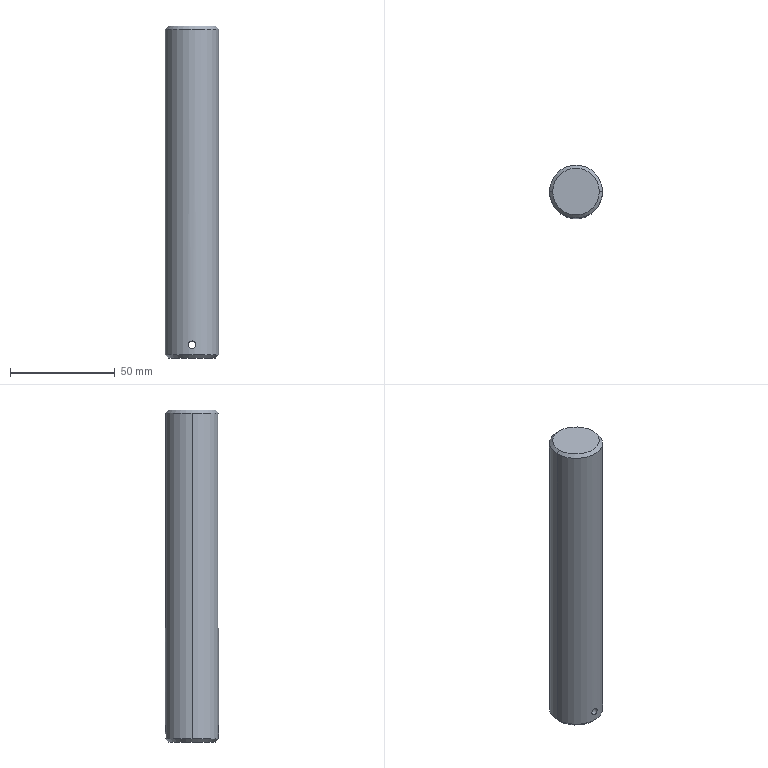Part | SolidWorks | features Chamfer 1, Extrusion 1, ICE 1 | 1 solid | 10 faces | box 25.4 x 25.4 x 158.75 mm | volume 80008 mm3 | cylinder 4 | cone 4 | plane 2 | commonest cylinder face diameters 3.57 x2 25.4 x2
STEP:
#1=CARTESIAN_POINT('',(0.,-12.7,4.565));
#2=VERTEX_POINT('',#1);
#3=CARTESIAN_POINT('',(0.,-12.7,8.135));
#4=VERTEX_POINT('',#3);
#5=CARTESIAN_POINT('',(0.,-12.7,4.565));
#6=CARTESIAN_POINT('',(-0.2331,-12.7,4.565));
#7=CARTESIAN_POINT('',(-0.4682,-12.693,4.612));
#8=CARTESIAN_POINT('',(-0.8979,-12.67,4.79));
#9=CARTESIAN_POINT('',(-1.097,-12.654,4.923));
#10=CARTESIAN_POINT('',(-1.344,-12.629,5.169));
#11=CARTESIAN_POINT('',(-1.419,-12.621,5.261));
#12=CARTESIAN_POINT('',(-1.549,-12.605,5.455));
#13=CARTESIAN_POINT('',(-1.603,-12.598,5.557));
#14=CARTESIAN_POINT('',(-1.693,-12.587,5.773));
#15=CARTESIAN_POINT('',(-1.728,-12.582,5.886));
#16=CARTESIAN_POINT('',(-1.773,-12.576,6.115));
#17=CARTESIAN_POINT('',(-1.785,-12.574,6.231));
#18=CARTESIAN_POINT('',(-1.785,-12.574,6.467));
#19=CARTESIAN_POINT('',(-1.774,-12.576,6.583));
#20=CARTESIAN_POINT('',(-1.728,-12.582,6.811));
#21=CARTESIAN_POINT('',(-1.694,-12.587,6.925));
#22=CARTESIAN_POINT('',(-1.605,-12.598,7.141));
#23=CARTESIAN_POINT('',(-1.55,-12.605,7.243));
#24=CARTESIAN_POINT('',(-1.42,-12.62,7.437));
#25=CARTESIAN_POINT('',(-1.345,-12.629,7.529));
#26=CARTESIAN_POINT('',(-1.099,-12.653,7.776));
#27=CARTESIAN_POINT('',(-0.9,-12.67,7.909));
#28=CARTESIAN_POINT('',(-0.4707,-12.693,8.087));
#29=CARTESIAN_POINT('',(-0.2361,-12.7,8.135));
#30=CARTESIAN_POINT('',(0.,-12.7,8.135));
#31=B_SPLINE_CURVE_WITH_KNOTS('',3,(#5,#6,#7,#8,#9,#10,#11,#12,#13,#14,#15,#16,#17,#18,#19,#20,#21,#22,#23,#24,#25,#26,#27,#28,#29,#30),.UNSPECIFIED.,.F.,.F.,(4,2,2,2,2,2,2,2,2,2,2,2,4),(0.005588,0.006286,0.006984,0.007333,0.007682,0.008032,0.008381,0.00873,0.009079,0.009428,0.009777,0.01048,0.01117),.UNSPECIFIED.);
#32=EDGE_CURVE('',#2,#4,#31,.T.);
#33=ORIENTED_EDGE('',*,*,#32,.F.);
#34=CARTESIAN_POINT('',(0.,12.7,4.565));
#35=VERTEX_POINT('',#34);
#36=CARTESIAN_POINT('',(0.,-12.7,4.565));
#37=DIRECTION('',(0.,1.,0.));
#38=VECTOR('',#37,1000.);
#39=LINE('',#36,#38);
#40=EDGE_CURVE('',#2,#35,#39,.T.);
#41=ORIENTED_EDGE('',*,*,#40,.T.);
#42=CARTESIAN_POINT('',(0.,12.7,8.135));
#43=VERTEX_POINT('',#42);
#44=CARTESIAN_POINT('',(0.,12.7,8.135));
#45=CARTESIAN_POINT('',(-0.1181,12.7,8.135));
#46=CARTESIAN_POINT('',(-0.2342,12.698,8.123));
#47=CARTESIAN_POINT('',(-0.4625,12.692,8.078));
#48=CARTESIAN_POINT('',(-0.576,12.687,8.044));
#49=CARTESIAN_POINT('',(-0.7921,12.676,7.954));
#50=CARTESIAN_POINT('',(-0.8946,12.669,7.899));
#51=CARTESIAN_POINT('',(-1.089,12.654,7.769));
#52=CARTESIAN_POINT('',(-1.18,12.645,7.694));
#53=CARTESIAN_POINT('',(-1.427,12.621,7.447));
#54=CARTESIAN_POINT('',(-1.56,12.604,7.248));
#55=CARTESIAN_POINT('',(-1.738,12.581,6.819));
#56=CARTESIAN_POINT('',(-1.785,12.574,6.584));
#57=CARTESIAN_POINT('',(-1.785,12.574,6.234));
#58=CARTESIAN_POINT('',(-1.773,12.576,6.116));
#59=CARTESIAN_POINT('',(-1.728,12.582,5.887));
#60=CARTESIAN_POINT('',(-1.694,12.587,5.775));
#61=CARTESIAN_POINT('',(-1.604,12.598,5.559));
#62=CARTESIAN_POINT('',(-1.549,12.605,5.455));
#63=CARTESIAN_POINT('',(-1.419,12.621,5.261));
#64=CARTESIAN_POINT('',(-1.345,12.629,5.171));
#65=CARTESIAN_POINT('',(-1.179,12.645,5.005));
#66=CARTESIAN_POINT('',(-1.089,12.654,4.931));
#67=CARTESIAN_POINT('',(-0.8958,12.669,4.802));
#68=CARTESIAN_POINT('',(-0.7914,12.676,4.746));
#69=CARTESIAN_POINT('',(-0.5753,12.687,4.656));
#70=CARTESIAN_POINT('',(-0.4641,12.692,4.622));
#71=CARTESIAN_POINT('',(-0.235,12.698,4.577));
#72=CARTESIAN_POINT('',(-0.1166,12.7,4.565));
#73=CARTESIAN_POINT('',(0.,12.7,4.565));
#74=B_SPLINE_CURVE_WITH_KNOTS('',3,(#44,#45,#46,#47,#48,#49,#50,#51,#52,#53,#54,#55,#56,#57,#58,#59,#60,#61,#62,#63,#64,#65,#66,#67,#68,#69,#70,#71,#72,#73),.UNSPECIFIED.,.F.,.F.,(4,2,2,2,2,2,2,2,2,2,2,2,2,2,4),(0.,0.0003492,0.0006985,0.001048,0.001397,0.002095,0.002794,0.003143,0.003492,0.003842,0.004191,0.00454,0.004889,0.005238,0.005588),.UNSPECIFIED.);
#75=EDGE_CURVE('',#43,#35,#74,.T.);
#76=ORIENTED_EDGE('',*,*,#75,.F.);
#77=CARTESIAN_POINT('',(0.,-12.7,8.135));
#78=DIRECTION('',(0.,1.,0.));
#79=VECTOR('',#78,1000.);
#80=LINE('',#77,#79);
#81=EDGE_CURVE('',#4,#43,#80,.T.);
#82=ORIENTED_EDGE('',*,*,#81,.F.);
#83=EDGE_LOOP('',(#33,#41,#76,#82));
#84=FACE_OUTER_BOUND('',#83,.T.);
#85=CARTESIAN_POINT('',(0.,-12.7,6.35));
#86=DIRECTION('',(0.,1.,0.));
#87=DIRECTION('',(0.,0.,1.));
#88=AXIS2_PLACEMENT_3D('',#85,#86,#87);
#89=CYLINDRICAL_SURFACE('',#88,1.785);
#90=ADVANCED_FACE('',(#84),#89,.F.);
#91=CARTESIAN_POINT('',(11.176,0.,158.75));
#92=VERTEX_POINT('',#91);
#93=CARTESIAN_POINT('',(-11.176,0.,158.75));
#94=VERTEX_POINT('',#93);
#95=CARTESIAN_POINT('',(0.,0.,158.75));
#96=DIRECTION('',(0.,0.,1.));
#97=DIRECTION('',(1.,0.,0.));
#98=AXIS2_PLACEMENT_3D('',#95,#96,#97);
#99=CIRCLE('',#98,11.176);
#100=EDGE_CURVE('',#92,#94,#99,.T.);
#101=ORIENTED_EDGE('',*,*,#100,.F.);
#102=CARTESIAN_POINT('',(12.7,0.,157.226));
#103=VERTEX_POINT('',#102);
#104=CARTESIAN_POINT('',(11.176,0.,158.75));
#105=DIRECTION('',(0.7071,0.,-0.7071));
#106=VECTOR('',#105,1000.);
#107=LINE('',#104,#106);
#108=EDGE_CURVE('',#92,#103,#107,.T.);
#109=ORIENTED_EDGE('',*,*,#108,.T.);
#110=CARTESIAN_POINT('',(-12.7,0.,157.226));
#111=VERTEX_POINT('',#110);
#112=CARTESIAN_POINT('',(0.,0.,157.226));
#113=DIRECTION('',(0.,0.,-1.));
#114=DIRECTION('',(1.,0.,0.));
#115=AXIS2_PLACEMENT_3D('',#112,#113,#114);
#116=CIRCLE('',#115,12.7);
#117=EDGE_CURVE('',#111,#103,#116,.T.);
#118=ORIENTED_EDGE('',*,*,#117,.F.);
#119=CARTESIAN_POINT('',(-11.176,0.,158.75));
#120=DIRECTION('',(-0.7071,0.,-0.7071));
#121=VECTOR('',#120,1000.);
#122=LINE('',#119,#121);
#123=EDGE_CURVE('',#94,#111,#122,.T.);
#124=ORIENTED_EDGE('',*,*,#123,.F.);
#125=EDGE_LOOP('',(#101,#109,#118,#124));
#126=FACE_OUTER_BOUND('',#125,.T.);
#127=CARTESIAN_POINT('',(0.,0.,158.75));
#128=DIRECTION('',(0.,0.,-1.));
#129=DIRECTION('',(-1.,0.,0.));
#130=AXIS2_PLACEMENT_3D('',#127,#128,#129);
#131=CONICAL_SURFACE('',#130,11.176,0.7854);
#132=ADVANCED_FACE('',(#126),#131,.T.);
#133=CARTESIAN_POINT('',(-11.176,0.,0.));
#134=VERTEX_POINT('',#133);
#135=CARTESIAN_POINT('',(11.176,0.,0.));
#136=VERTEX_POINT('',#135);
#137=CARTESIAN_POINT('',(0.,0.,0.));
#138=DIRECTION('',(0.,0.,-1.));
#139=DIRECTION('',(1.,0.,0.));
#140=AXIS2_PLACEMENT_3D('',#137,#138,#139);
#141=CIRCLE('',#140,11.176);
#142=EDGE_CURVE('',#134,#136,#141,.T.);
#143=ORIENTED_EDGE('',*,*,#142,.F.);
#144=CARTESIAN_POINT('',(-12.7,0.,1.524));
#145=VERTEX_POINT('',#144);
#146=CARTESIAN_POINT('',(-12.7,0.,1.524));
#147=DIRECTION('',(-0.7071,0.,0.7071));
#148=VECTOR('',#147,1000.);
#149=LINE('',#146,#148);
#150=EDGE_CURVE('',#134,#145,#149,.T.);
#151=ORIENTED_EDGE('',*,*,#150,.T.);
#152=CARTESIAN_POINT('',(12.7,0.,1.524));
#153=VERTEX_POINT('',#152);
#154=CARTESIAN_POINT('',(0.,0.,1.524));
#155=DIRECTION('',(0.,0.,1.));
#156=DIRECTION('',(1.,0.,0.));
#157=AXIS2_PLACEMENT_3D('',#154,#155,#156);
#158=CIRCLE('',#157,12.7);
#159=EDGE_CURVE('',#153,#145,#158,.T.);
#160=ORIENTED_EDGE('',*,*,#159,.F.);
#161=CARTESIAN_POINT('',(12.7,0.,1.524));
#162=DIRECTION('',(0.7071,0.,0.7071));
#163=VECTOR('',#162,1000.);
#164=LINE('',#161,#163);
#165=EDGE_CURVE('',#136,#153,#164,.T.);
#166=ORIENTED_EDGE('',*,*,#165,.F.);
#167=EDGE_LOOP('',(#143,#151,#160,#166));
#168=FACE_OUTER_BOUND('',#167,.T.);
#169=CARTESIAN_POINT('',(0.,0.,1.524));
#170=DIRECTION('',(0.,0.,1.));
#171=DIRECTION('',(1.,0.,0.));
#172=AXIS2_PLACEMENT_3D('',#169,#170,#171);
#173=CONICAL_SURFACE('',#172,12.7,0.7854);
#174=ADVANCED_FACE('',(#168),#173,.T.);
#175=ORIENTED_EDGE('',*,*,#75,.T.);
#176=CARTESIAN_POINT('',(0.,12.7,4.565));
#177=CARTESIAN_POINT('',(0.2331,12.7,4.565));
#178=CARTESIAN_POINT('',(0.4682,12.693,4.612));
#179=CARTESIAN_POINT('',(0.8979,12.67,4.79));
#180=CARTESIAN_POINT('',(1.097,12.654,4.923));
#181=CARTESIAN_POINT('',(1.344,12.629,5.169));
#182=CARTESIAN_POINT('',(1.419,12.621,5.261));
#183=CARTESIAN_POINT('',(1.549,12.605,5.455));
#184=CARTESIAN_POINT('',(1.603,12.598,5.557));
#185=CARTESIAN_POINT('',(1.693,12.587,5.773));
#186=CARTESIAN_POINT('',(1.728,12.582,5.886));
#187=CARTESIAN_POINT('',(1.773,12.576,6.115));
#188=CARTESIAN_POINT('',(1.785,12.574,6.231));
#189=CARTESIAN_POINT('',(1.785,12.574,6.467));
#190=CARTESIAN_POINT('',(1.774,12.576,6.583));
#191=CARTESIAN_POINT('',(1.728,12.582,6.811));
#192=CARTESIAN_POINT('',(1.694,12.587,6.925));
#193=CARTESIAN_POINT('',(1.605,12.598,7.141));
#194=CARTESIAN_POINT('',(1.55,12.605,7.243));
#195=CARTESIAN_POINT('',(1.42,12.62,7.437));
#196=CARTESIAN_POINT('',(1.345,12.629,7.529));
#197=CARTESIAN_POINT('',(1.099,12.653,7.776));
#198=CARTESIAN_POINT('',(0.9,12.67,7.909));
#199=CARTESIAN_POINT('',(0.4707,12.693,8.087));
#200=CARTESIAN_POINT('',(0.2361,12.7,8.135));
#201=CARTESIAN_POINT('',(0.,12.7,8.135));
#202=B_SPLINE_CURVE_WITH_KNOTS('',3,(#176,#177,#178,#179,#180,#181,#182,#183,#184,#185,#186,#187,#188,#189,#190,#191,#192,#193,#194,#195,#196,#197,#198,#199,#200,#201),.UNSPECIFIED.,.F.,.F.,(4,2,2,2,2,2,2,2,2,2,2,2,4),(0.005588,0.006286,0.006984,0.007333,0.007682,0.008032,0.008381,0.00873,0.009079,0.009428,0.009777,0.01048,0.01117),.UNSPECIFIED.);
#203=EDGE_CURVE('',#35,#43,#202,.T.);
#204=ORIENTED_EDGE('',*,*,#203,.T.);
#205=EDGE_LOOP('',(#175,#204));
#206=FACE_BOUND('',#205,.T.);
#207=ORIENTED_EDGE('',*,*,#117,.T.);
#208=CARTESIAN_POINT('',(12.7,0.,158.75));
#209=DIRECTION('',(0.,0.,-1.));
#210=VECTOR('',#209,1000.);
#211=LINE('',#208,#210);
#212=EDGE_CURVE('',#103,#153,#211,.T.);
#213=ORIENTED_EDGE('',*,*,#212,.T.);
#214=ORIENTED_EDGE('',*,*,#159,.T.);
#215=CARTESIAN_POINT('',(-12.7,0.,158.75));
#216=DIRECTION('',(0.,0.,-1.));
#217=VECTOR('',#216,1000.);
#218=LINE('',#215,#217);
#219=EDGE_CURVE('',#111,#145,#218,.T.);
#220=ORIENTED_EDGE('',*,*,#219,.F.);
#221=EDGE_LOOP('',(#207,#213,#214,#220));
#222=FACE_OUTER_BOUND('',#221,.T.);
#223=CARTESIAN_POINT('',(0.,0.,158.75));
#224=DIRECTION('',(0.,0.,-1.));
#225=DIRECTION('',(-1.,0.,0.));
#226=AXIS2_PLACEMENT_3D('',#223,#224,#225);
#227=CYLINDRICAL_SURFACE('',#226,12.7);
#228=ADVANCED_FACE('',(#206,#222),#227,.T.);
#229=ORIENTED_EDGE('',*,*,#212,.F.);
#230=CARTESIAN_POINT('',(0.,0.,157.226));
#231=DIRECTION('',(0.,0.,-1.));
#232=DIRECTION('',(1.,0.,0.));
#233=AXIS2_PLACEMENT_3D('',#230,#231,#232);
#234=CIRCLE('',#233,12.7);
#235=EDGE_CURVE('',#103,#111,#234,.T.);
#236=ORIENTED_EDGE('',*,*,#235,.T.);
#237=ORIENTED_EDGE('',*,*,#219,.T.);
#238=CARTESIAN_POINT('',(0.,0.,1.524));
#239=DIRECTION('',(0.,0.,1.));
#240=DIRECTION('',(1.,0.,0.));
#241=AXIS2_PLACEMENT_3D('',#238,#239,#240);
#242=CIRCLE('',#241,12.7);
#243=EDGE_CURVE('',#145,#153,#242,.T.);
#244=ORIENTED_EDGE('',*,*,#243,.T.);
#245=EDGE_LOOP('',(#229,#236,#237,#244));
#246=FACE_OUTER_BOUND('',#245,.T.);
#247=CARTESIAN_POINT('',(0.,-12.7,8.135));
#248=CARTESIAN_POINT('',(0.1181,-12.7,8.135));
#249=CARTESIAN_POINT('',(0.2342,-12.698,8.123));
#250=CARTESIAN_POINT('',(0.4625,-12.692,8.078));
#251=CARTESIAN_POINT('',(0.576,-12.687,8.044));
#252=CARTESIAN_POINT('',(0.7921,-12.676,7.954));
#253=CARTESIAN_POINT('',(0.8946,-12.669,7.899));
#254=CARTESIAN_POINT('',(1.089,-12.654,7.769));
#255=CARTESIAN_POINT('',(1.18,-12.645,7.694));
#256=CARTESIAN_POINT('',(1.427,-12.621,7.447));
#257=CARTESIAN_POINT('',(1.56,-12.604,7.248));
#258=CARTESIAN_POINT('',(1.738,-12.581,6.819));
#259=CARTESIAN_POINT('',(1.785,-12.574,6.584));
#260=CARTESIAN_POINT('',(1.785,-12.574,6.234));
#261=CARTESIAN_POINT('',(1.773,-12.576,6.116));
#262=CARTESIAN_POINT('',(1.728,-12.582,5.887));
#263=CARTESIAN_POINT('',(1.694,-12.587,5.775));
#264=CARTESIAN_POINT('',(1.604,-12.598,5.559));
#265=CARTESIAN_POINT('',(1.549,-12.605,5.455));
#266=CARTESIAN_POINT('',(1.419,-12.621,5.261));
#267=CARTESIAN_POINT('',(1.345,-12.629,5.171));
#268=CARTESIAN_POINT('',(1.179,-12.645,5.005));
#269=CARTESIAN_POINT('',(1.089,-12.654,4.931));
#270=CARTESIAN_POINT('',(0.8958,-12.669,4.802));
#271=CARTESIAN_POINT('',(0.7914,-12.676,4.746));
#272=CARTESIAN_POINT('',(0.5753,-12.687,4.656));
#273=CARTESIAN_POINT('',(0.4641,-12.692,4.622));
#274=CARTESIAN_POINT('',(0.235,-12.698,4.577));
#275=CARTESIAN_POINT('',(0.1166,-12.7,4.565));
#276=CARTESIAN_POINT('',(0.,-12.7,4.565));
#277=B_SPLINE_CURVE_WITH_KNOTS('',3,(#247,#248,#249,#250,#251,#252,#253,#254,#255,#256,#257,#258,#259,#260,#261,#262,#263,#264,#265,#266,#267,#268,#269,#270,#271,#272,#273,#274,#275,#276),.UNSPECIFIED.,.F.,.F.,(4,2,2,2,2,2,2,2,2,2,2,2,2,2,4),(0.,0.0003492,0.0006985,0.001048,0.001397,0.002095,0.002794,0.003143,0.003492,0.003842,0.004191,0.00454,0.004889,0.005238,0.005588),.UNSPECIFIED.);
#278=EDGE_CURVE('',#4,#2,#277,.T.);
#279=ORIENTED_EDGE('',*,*,#278,.T.);
#280=ORIENTED_EDGE('',*,*,#32,.T.);
#281=EDGE_LOOP('',(#279,#280));
#282=FACE_BOUND('',#281,.T.);
#283=CARTESIAN_POINT('',(0.,0.,158.75));
#284=DIRECTION('',(0.,0.,-1.));
#285=DIRECTION('',(-1.,0.,0.));
#286=AXIS2_PLACEMENT_3D('',#283,#284,#285);
#287=CYLINDRICAL_SURFACE('',#286,12.7);
#288=ADVANCED_FACE('',(#246,#282),#287,.T.);
#289=CARTESIAN_POINT('',(0.,0.,158.75));
#290=DIRECTION('',(0.,0.,1.));
#291=DIRECTION('',(1.,0.,0.));
#292=AXIS2_PLACEMENT_3D('',#289,#290,#291);
#293=CIRCLE('',#292,11.176);
#294=EDGE_CURVE('',#94,#92,#293,.T.);
#295=ORIENTED_EDGE('',*,*,#294,.T.);
#296=ORIENTED_EDGE('',*,*,#100,.T.);
#297=EDGE_LOOP('',(#295,#296));
#298=FACE_OUTER_BOUND('',#297,.T.);
#299=CARTESIAN_POINT('',(0.,0.,158.75));
#300=DIRECTION('',(0.,0.,1.));
#301=DIRECTION('',(1.,0.,0.));
#302=AXIS2_PLACEMENT_3D('',#299,#300,#301);
#303=PLANE('',#302);
#304=ADVANCED_FACE('',(#298),#303,.T.);
#305=CARTESIAN_POINT('',(0.,0.,0.));
#306=DIRECTION('',(0.,0.,-1.));
#307=DIRECTION('',(1.,0.,0.));
#308=AXIS2_PLACEMENT_3D('',#305,#306,#307);
#309=CIRCLE('',#308,11.176);
#310=EDGE_CURVE('',#136,#134,#309,.T.);
#311=ORIENTED_EDGE('',*,*,#310,.T.);
#312=ORIENTED_EDGE('',*,*,#142,.T.);
#313=EDGE_LOOP('',(#311,#312));
#314=FACE_OUTER_BOUND('',#313,.T.);
#315=CARTESIAN_POINT('',(0.,0.,0.));
#316=DIRECTION('',(0.,0.,1.));
#317=DIRECTION('',(1.,0.,0.));
#318=AXIS2_PLACEMENT_3D('',#315,#316,#317);
#319=PLANE('',#318);
#320=ADVANCED_FACE('',(#314),#319,.F.);
#321=ORIENTED_EDGE('',*,*,#150,.F.);
#322=ORIENTED_EDGE('',*,*,#310,.F.);
#323=ORIENTED_EDGE('',*,*,#165,.T.);
#324=ORIENTED_EDGE('',*,*,#243,.F.);
#325=EDGE_LOOP('',(#321,#322,#323,#324));
#326=FACE_OUTER_BOUND('',#325,.T.);
#327=CARTESIAN_POINT('',(0.,0.,1.524));
#328=DIRECTION('',(0.,0.,1.));
#329=DIRECTION('',(1.,0.,0.));
#330=AXIS2_PLACEMENT_3D('',#327,#328,#329);
#331=CONICAL_SURFACE('',#330,12.7,0.7854);
#332=ADVANCED_FACE('',(#326),#331,.T.);
#333=ORIENTED_EDGE('',*,*,#108,.F.);
#334=ORIENTED_EDGE('',*,*,#294,.F.);
#335=ORIENTED_EDGE('',*,*,#123,.T.);
#336=ORIENTED_EDGE('',*,*,#235,.F.);
#337=EDGE_LOOP('',(#333,#334,#335,#336));
#338=FACE_OUTER_BOUND('',#337,.T.);
#339=CARTESIAN_POINT('',(0.,0.,158.75));
#340=DIRECTION('',(0.,0.,-1.));
#341=DIRECTION('',(-1.,0.,0.));
#342=AXIS2_PLACEMENT_3D('',#339,#340,#341);
#343=CONICAL_SURFACE('',#342,11.176,0.7854);
#344=ADVANCED_FACE('',(#338),#343,.T.);
#345=ORIENTED_EDGE('',*,*,#40,.F.);
#346=ORIENTED_EDGE('',*,*,#278,.F.);
#347=ORIENTED_EDGE('',*,*,#81,.T.);
#348=ORIENTED_EDGE('',*,*,#203,.F.);
#349=EDGE_LOOP('',(#345,#346,#347,#348));
#350=FACE_OUTER_BOUND('',#349,.T.);
#351=CARTESIAN_POINT('',(0.,-12.7,6.35));
#352=DIRECTION('',(0.,1.,0.));
#353=DIRECTION('',(0.,0.,1.));
#354=AXIS2_PLACEMENT_3D('',#351,#352,#353);
#355=CYLINDRICAL_SURFACE('',#354,1.785);
#356=ADVANCED_FACE('',(#350),#355,.F.);
#357=CLOSED_SHELL('',(#90,#132,#174,#228,#288,#304,#320,#332,#344,#356));
#358=MANIFOLD_SOLID_BREP('',#357);
#359=CARTESIAN_POINT('',(0.,0.,0.));
#360=DIRECTION('',(0.,0.,1.));
#361=DIRECTION('',(1.,0.,0.));
#362=AXIS2_PLACEMENT_3D('',#359,#360,#361);
#363=(LENGTH_UNIT()NAMED_UNIT(*)SI_UNIT(.MILLI.,.METRE.));
#364=UNCERTAINTY_MEASURE_WITH_UNIT(LENGTH_MEASURE(0.00001),#363,'','');
#365=(NAMED_UNIT(*)PLANE_ANGLE_UNIT()SI_UNIT($,.RADIAN.));
#366=(NAMED_UNIT(*)SI_UNIT($,.STERADIAN.)SOLID_ANGLE_UNIT());
#367=(GEOMETRIC_REPRESENTATION_CONTEXT(3)GLOBAL_UNCERTAINTY_ASSIGNED_CONTEXT((#364))GLOBAL_UNIT_ASSIGNED_CONTEXT((#363,#365,#366))REPRESENTATION_CONTEXT('',''));
#368=ADVANCED_BREP_SHAPE_REPRESENTATION('',(#358,#362),#367);